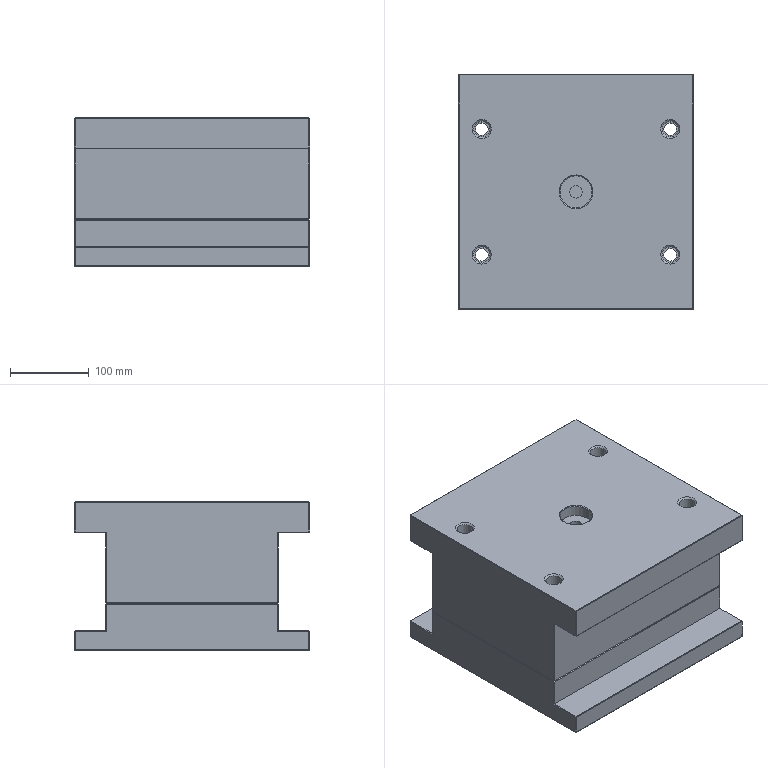NC program | NX | posted with a generic post | part box 300 x 300 x 190 mm
Lines 1 to 902 of 34829:
N10 G17 G21 G94 G90
(CAVITY_MILL_COPY_1 , TOOL : D25R5)
N12 T02 M6
N14 G54
N16 G17 G0 G90 X-7.201 Y-12.74 S1000 M3
N18 G43 Z30. H2
N20 Z1.5
N22 G94 G1 X-6.125 Y-13.304 Z1.436 F1000.
N24 X-4.712 Y-13.868 Z1.357
N26 X-3.248 Y-14.282 Z1.277
N28 X-2.184 Y-14.483 Z1.22
N30 X-1.089 Y-14.606 Z1.162
N32 X0.012 Y-14.646 Z1.105
N34 X1.113 Y-14.604 Z1.047
N36 X2.188 Y-14.482 Z0.99
N38 X3.607 Y-14.195 Z0.914
N40 X4.99 Y-13.77 Z0.838
N42 X6.325 Y-13.211 Z0.763
N44 X7.597 Y-12.522 Z0.687
N46 X8.796 Y-11.711 Z0.611
N48 X9.909 Y-10.786 Z0.535
N50 X10.925 Y-9.755 Z0.459
N52 X11.834 Y-8.629 Z0.383
N54 X12.628 Y-7.419 Z0.308
N56 X13.299 Y-6.137 Z0.232
N58 X13.839 Y-4.795 Z0.156
N60 X14.245 Y-3.405 Z0.08
N62 X14.512 Y-1.983 Z0.004
N64 X14.636 Y-0.541 Z-0.072
N66 Y0. Z-0.1
N68 X4.886
N70 G3 X0. Y4.886 R4.886 F2000.
N72 X4.886 Y0. R-4.886
N74 G1 X14.636
N76 G3 X0. Y14.636 R14.636
N78 X14.636 Y0. R-14.636
N80 G1 X24.386
N82 G3 X0. Y24.386 R24.386
N84 X24.386 Y0. R-24.386
N86 G1 X34.136
N88 G3 X0. Y34.136 R34.136
N90 X34.136 Y0. R-34.136
N92 G1 X43.886
N94 G3 X0. Y43.886 R43.886
N96 X43.886 Y0. R-43.886
N98 X43.386 Y0.866 R1.
N100 G1 Z1.4
N102 G0 X-11.531 Y-7.454
N104 G1 X-11.121 Y-8.085 Z1.361 F1000.
N106 X-10.205 Y-9.214 Z1.284
N108 X-9.175 Y-10.24 Z1.208
N110 X-8.042 Y-11.152 Z1.132
N112 X-6.819 Y-11.939 Z1.056
N114 X-5.52 Y-12.593 Z0.979
N116 X-4.159 Y-13.105 Z0.903
N118 X-2.751 Y-13.471 Z0.827
N120 X-1.716 Y-13.642 Z0.772
N122 X-0.443 Y-13.742 Z0.705
N124 X0.834 Y-13.724 Z0.638
N126 X1.877 Y-13.621 Z0.583
N128 X3.326 Y-13.341 Z0.506
N130 X4.736 Y-12.908 Z0.429
N132 X6.092 Y-12.326 Z0.351
N134 X7.378 Y-11.602 Z0.274
N136 X8.579 Y-10.745 Z0.197
N138 X9.681 Y-9.764 Z0.119
N140 X10.671 Y-8.67 Z0.042
N142 X11.539 Y-7.477 Z-0.035
N144 X12.273 Y-6.197 Z-0.113
N146 X12.867 Y-4.846 Z-0.19
N148 X13.312 Y-3.44 Z-0.267
N150 X13.604 Y-1.994 Z-0.345
N152 X13.739 Y-0.524 Z-0.422
N154 Y0. Z-0.449
N156 X3.989
N158 G3 X0. Y3.989 R3.989 F2000.
N160 X3.989 Y0. R-3.989
N162 G1 X13.739
N164 G3 X0. Y13.739 R13.739
N166 X13.739 Y0. R-13.739
N168 G1 X23.489
N170 G3 X0. Y23.489 R23.489
N172 X23.489 Y0. R-23.489
N174 G1 X33.239
N176 G3 X0. Y33.239 R33.239
N178 X33.239 Y0. R-33.239
N180 G1 X42.989
N182 G3 X0. Y42.989 R42.989
N184 X42.989 Y0. R-42.989
N186 X42.489 Y0.866 R1.
N188 G1 Z1.051
N190 G0 X11.782 Y5.822
N192 G1 X11.396 Y6.583 Z1.006 F1000.
N194 X10.849 Y7.45 Z0.952
N196 X9.981 Y8.578 Z0.878
N198 X8.997 Y9.605 Z0.803
N200 X7.908 Y10.52 Z0.728
N202 X6.726 Y11.312 Z0.654
N204 X5.466 Y11.972 Z0.579
N206 X4.142 Y12.492 Z0.505
N208 X2.769 Y12.866 Z0.43
N210 X1.364 Y13.09 Z0.356
N212 X-0.057 Y13.16 Z0.281
N214 X-1.477 Y13.077 Z0.207
N216 X-2.88 Y12.842 Z0.132
N218 X-4.249 Y12.456 Z0.057
N220 X-5.569 Y11.924 Z-0.017
N222 X-6.823 Y11.254 Z-0.092
N224 X-7.998 Y10.451 Z-0.166
N226 X-9.079 Y9.527 Z-0.241
N228 X-10.055 Y8.491 Z-0.315
N230 X-10.912 Y7.357 Z-0.39
N232 X-11.452 Y6.484 Z-0.444
N234 X-12.017 Y5.366 Z-0.509
N236 X-12.473 Y4.199 Z-0.575
N238 X-12.816 Y2.993 Z-0.641
N240 X-13.042 Y1.761 Z-0.706
N242 X-13.151 Y0.513 Z-0.772
N244 Y0. Z-0.799
N246 X-3.401
N248 G3 X0. Y-3.401 R3.401 F2000.
N250 X-3.401 Y0. R-3.401
N252 G1 X-13.151
N254 G3 X0. Y-13.151 R13.151
N256 X-13.151 Y0. R-13.151
N258 G1 X-22.901
N260 G3 X0. Y-22.901 R22.901
N262 X-22.901 Y0. R-22.901
N264 G1 X-32.651
N266 G3 X0. Y-32.651 R32.651
N268 X-32.651 Y0. R-32.651
N270 G1 X-42.401
N272 G3 X0. Y-42.401 R42.401
N274 X-42.401 Y0. R-42.401
N276 X-41.901 Y-0.866 R1.
N278 G1 Z0.701
N280 G0 X4.519 Y-11.874
N282 G1 X5.691 Y-11.364 Z0.634 F1000.
N284 X6.88 Y-10.686 Z0.562
N286 X7.99 Y-9.884 Z0.491
N288 X9.006 Y-8.967 Z0.419
N290 X9.919 Y-7.946 Z0.347
N292 X10.716 Y-6.833 Z0.275
N294 X11.389 Y-5.641 Z0.204
N296 X11.929 Y-4.383 Z0.132
N298 X12.332 Y-3.075 Z0.06
N300 X12.591 Y-1.731 Z-0.012
N302 X12.704 Y-0.366 Z-0.083
N304 X12.67 Y1.002 Z-0.155
N306 X12.488 Y2.359 Z-0.227
N308 X12.162 Y3.689 Z-0.299
N310 X11.695 Y4.976 Z-0.37
N312 X11.092 Y6.205 Z-0.442
N314 X10.565 Y7.064 Z-0.495
N316 X9.769 Y8.129 Z-0.565
N318 X8.867 Y9.105 Z-0.634
N320 X7.867 Y9.981 Z-0.704
N322 X6.782 Y10.749 Z-0.774
N324 X5.622 Y11.398 Z-0.843
N326 X4.401 Y11.923 Z-0.913
N328 X3.131 Y12.317 Z-0.983
N330 X1.828 Y12.577 Z-1.052
N332 X0.504 Y12.699 Z-1.122
N334 X0. Z-1.148
N336 Y2.949
N338 G3 X-2.949 Y0. R2.949 F2000.
N340 X0. Y2.949 R-2.949
N342 G1 Y12.699
N344 G3 X-12.699 Y0. R12.699
N346 X0. Y12.699 R-12.699
N348 G1 Y22.449
N350 G3 X-22.449 Y0. R22.449
N352 X0. Y22.449 R-22.449
N354 G1 Y32.199
N356 G3 X-32.199 Y0. R32.199
N358 X0. Y32.199 R-32.199
N360 G1 Y41.949
N362 G3 X-41.949 Y0. R41.949
N364 X0. Y41.949 R-41.949
N366 X-0.866 Y41.449 R1.
N368 G1 Z0.352
N370 G0 X3.427 Y-11.844
N372 G1 X4.33 Y-11.561 Z0.302 F1000.
N374 X5.55 Y-11.027 Z0.232
N376 X6.706 Y-10.365 Z0.163
N378 X7.783 Y-9.582 Z0.093
N380 X8.771 Y-8.687 Z0.023
N382 X9.656 Y-7.692 Z-0.047
N384 X10.428 Y-6.607 Z-0.117
N386 X11.079 Y-5.445 Z-0.187
N388 X11.601 Y-4.219 Z-0.256
N390 X11.988 Y-2.945 Z-0.326
N392 X12.236 Y-1.636 Z-0.396
N394 X12.341 Y-0.308 Z-0.466
N396 X12.302 Y1.024 Z-0.536
N398 X12.12 Y2.343 Z-0.605
N400 X11.797 Y3.635 Z-0.675
N402 X11.337 Y4.885 Z-0.745
N404 X10.745 Y6.078 Z-0.815
N406 X10.221 Y6.923 Z-0.867
N408 X9.448 Y7.946 Z-0.934
N410 X8.573 Y8.883 Z-1.001
N412 X7.605 Y9.724 Z-1.068
N414 X6.555 Y10.46 Z-1.136
N416 X5.435 Y11.084 Z-1.203
N418 X4.256 Y11.588 Z-1.27
N420 X3.031 Y11.967 Z-1.337
N422 X1.774 Y12.217 Z-1.404
N424 X0.497 Y12.335 Z-1.472
N426 X0. Z-1.498
N428 Y2.585
N430 G3 X-2.585 Y0. R2.585 F2000.
N432 X0. Y2.585 R-2.585
N434 G1 Y12.335
N436 G3 X-12.335 Y0. R12.335
N438 X0. Y12.335 R-12.335
N440 G1 Y22.085
N442 G3 X-22.085 Y0. R22.085
N444 X0. Y22.085 R-22.085
N446 G1 Y31.835
N448 G3 X-31.835 Y0. R31.835
N450 X0. Y31.835 R-31.835
N452 G1 Y41.585
N454 G3 X-41.585 Y0. R41.585
N456 X0. Y41.585 R-41.585
N458 X-0.866 Y41.085 R1.
N460 G1 Z0.002
N462 G0 X2.506 Y-11.76
N464 G1 X3.075 Y-11.644 Z-0.028 F1000.
N466 X4.384 Y-11.217 Z-0.1
N468 X5.637 Y-10.643 Z-0.172
N470 X6.816 Y-9.929 Z-0.245
N472 X7.905 Y-9.086 Z-0.317
N474 X8.891 Y-8.123 Z-0.389
N476 X9.761 Y-7.055 Z-0.461
N478 X10.503 Y-5.894 Z-0.534
N480 X11.107 Y-4.655 Z-0.606
N482 X11.566 Y-3.356 Z-0.678
N484 X11.874 Y-2.013 Z-0.75
N486 X12.026 Y-0.644 Z-0.822
N488 X12.021 Y0.734 Z-0.895
N490 X11.858 Y2.102 Z-0.967
N492 X11.541 Y3.443 Z-1.039
N494 X11.072 Y4.739 Z-1.111
N496 X10.458 Y5.972 Z-1.183
N498 X9.937 Y6.804 Z-1.235
N500 X9.183 Y7.792 Z-1.3
N502 X8.33 Y8.698 Z-1.365
N504 X7.389 Y9.51 Z-1.43
N506 X6.369 Y10.221 Z-1.496
N508 X5.281 Y10.824 Z-1.561
N510 X4.137 Y11.311 Z-1.626
N512 X2.949 Y11.677 Z-1.691
N514 X1.729 Y11.919 Z-1.756
N516 X0.491 Y12.033 Z-1.821
N518 X0. Z-1.847
N520 Y2.283
N522 G3 X-2.283 Y0. R2.283 F2000.
N524 X0. Y2.283 R-2.283
N526 G1 Y12.033
N528 G3 X-12.033 Y0. R12.033
N530 X0. Y12.033 R-12.033
N532 G1 Y21.783
N534 G3 X-21.783 Y0. R21.783
N536 X0. Y21.783 R-21.783
N538 G1 Y31.533
N540 G3 X-31.533 Y0. R31.533
N542 X0. Y31.533 R-31.533
N544 G1 Y41.283
N546 G3 X-41.283 Y0. R41.283
N548 X0. Y41.283 R-41.283
N550 X-0.866 Y40.783 R1.
N552 G1 Z-0.347
N554 G0 X1.73 Y-11.662
N556 G1 X3.024 Y-11.397 Z-0.416 F1000.
N558 X4.308 Y-10.977 Z-0.487
N560 X5.535 Y-10.412 Z-0.558
N562 X6.689 Y-9.711 Z-0.629
N564 X7.756 Y-8.882 Z-0.699
N566 X8.72 Y-7.937 Z-0.77
N568 X9.571 Y-6.888 Z-0.841
N570 X10.296 Y-5.748 Z-0.912
N572 X10.886 Y-4.533 Z-0.983
N574 X11.333 Y-3.258 Z-1.053
N576 X11.631 Y-1.941 Z-1.124
N578 X11.776 Y-0.598 Z-1.195
N580 X11.768 Y0.752 Z-1.266
N582 X11.604 Y2.093 Z-1.337
N584 X11.289 Y3.406 Z-1.407
N586 X10.825 Y4.675 Z-1.478
N588 X10.22 Y5.882 Z-1.549
N590 X9.701 Y6.703 Z-1.6
N592 X8.863 Y7.778 Z-1.671
N594 X7.907 Y8.748 Z-1.743
N596 X6.845 Y9.602 Z-1.814
N598 X5.691 Y10.327 Z-1.885
N600 X4.462 Y10.915 Z-1.957
N602 X3.173 Y11.357 Z-2.028
N604 X1.841 Y11.647 Z-2.1
N606 X0.486 Y11.782 Z-2.171
N608 X0. Z-2.196
N610 Y2.032
N612 G3 X-2.032 Y0. R2.032 F2000.
N614 X0. Y2.032 R-2.032
N616 G1 Y11.782
N618 G3 X-11.782 Y0. R11.782
N620 X0. Y11.782 R-11.782
N622 G1 Y21.532
N624 G3 X-21.532 Y0. R21.532
N626 X0. Y21.532 R-21.532
N628 G1 Y31.282
N630 G3 X-31.282 Y0. R31.282
N632 X0. Y31.282 R-31.282
N634 G1 Y41.032
N636 G3 X-41.032 Y0. R41.032
N638 X0. Y41.032 R-41.032
N640 X-0.866 Y40.532 R1.
N642 G1 Z-0.696
N644 G0 X-11.514 Y-1.073
N646 G1 X-11.463 Y-1.654 Z-0.727 F1000.
N648 X-11.208 Y-2.918 Z-0.795
N650 X-10.814 Y-4.146 Z-0.862
N652 X-10.286 Y-5.322 Z-0.93
N654 X-9.63 Y-6.433 Z-0.997
N656 X-8.856 Y-7.463 Z-1.065
N658 X-7.971 Y-8.402 Z-1.133
N660 X-6.987 Y-9.236 Z-1.2
N662 X-5.917 Y-9.955 Z-1.268
N664 X-4.774 Y-10.552 Z-1.335
N666 X-3.571 Y-11.017 Z-1.403
N668 X-2.324 Y-11.346 Z-1.47
N670 X-1.374 Y-11.499 Z-1.521
N672 X-0.427 Y-11.573 Z-1.571
N674 X0.523 Y-11.569 Z-1.62
N676 X1.481 Y-11.486 Z-1.671
N678 X2.809 Y-11.235 Z-1.742
N680 X4.099 Y-10.832 Z-1.813
N682 X5.333 Y-10.28 Z-1.883
N684 X6.494 Y-9.589 Z-1.954
N686 X7.567 Y-8.768 Z-2.025
N688 X8.536 Y-7.827 Z-2.096
N690 X9.39 Y-6.779 Z-2.167
N692 X10.116 Y-5.639 Z-2.237
N694 X10.704 Y-4.422 Z-2.308
N696 X11.146 Y-3.145 Z-2.379
N698 X11.436 Y-1.826 Z-2.45
N700 X11.571 Y-0.481 Z-2.521
N702 Y0. Z-2.546
N704 X1.821
N706 G3 X0. Y1.821 R1.821 F2000.
N708 X1.821 Y0. R-1.821
N710 G1 X11.571
N712 G3 X0. Y11.571 R11.571
N714 X11.571 Y0. R-11.571
N716 G1 X21.321
N718 G3 X0. Y21.321 R21.321
N720 X21.321 Y0. R-21.321
N722 G1 X31.071
N724 G3 X0. Y31.071 R31.071
N726 X31.071 Y0. R-31.071
N728 G1 X40.821
N730 G3 X0. Y40.821 R40.821
N732 X40.821 Y0. R-40.821
N734 X40.321 Y0.866 R1.
N736 G1 Z-1.046
N738 G0 X-11.39 Y-0.527
N740 G1 X-11.275 Y-1.726 Z-1.109 F1000.
N742 X-11.008 Y-2.989 Z-1.177
N744 X-10.6 Y-4.214 Z-1.244
N746 X-10.056 Y-5.385 Z-1.312
N748 X-9.383 Y-6.486 Z-1.38
N750 X-8.59 Y-7.505 Z-1.447
N752 X-7.686 Y-8.428 Z-1.515
N754 X-6.685 Y-9.242 Z-1.583
N756 X-5.598 Y-9.939 Z-1.65
N758 X-4.439 Y-10.507 Z-1.718
N760 X-3.223 Y-10.942 Z-1.786
N762 X-1.966 Y-11.236 Z-1.853
N764 X-1.019 Y-11.361 Z-1.903
N766 X-0.153 Y-11.405 Z-1.949
N768 X0.714 Y-11.384 Z-1.994
N770 X1.664 Y-11.284 Z-2.044
N772 X2.95 Y-11.018 Z-2.113
N774 X4.197 Y-10.606 Z-2.182
N776 X5.389 Y-10.053 Z-2.251
N778 X6.509 Y-9.367 Z-2.32
N780 X7.542 Y-8.557 Z-2.388
N782 X8.476 Y-7.633 Z-2.457
N784 X9.297 Y-6.608 Z-2.526
N786 X9.995 Y-5.496 Z-2.595
N788 X10.561 Y-4.31 Z-2.664
N790 X10.986 Y-3.068 Z-2.733
N792 X11.266 Y-1.784 Z-2.801
N794 X11.397 Y-0.478 Z-2.87
N796 Y0. Z-2.895
N798 X1.647
N800 G3 X0. Y1.647 R1.647 F2000.
N802 X1.647 Y0. R-1.647
N804 G1 X11.397
N806 G3 X0. Y11.397 R11.397
N808 X11.397 Y0. R-11.397
N810 G1 X21.147
N812 G3 X0. Y21.147 R21.147
N814 X21.147 Y0. R-21.147
N816 G1 X30.897
N818 G3 X0. Y30.897 R30.897
N820 X30.897 Y0. R-30.897
N822 G1 X40.647
N824 G3 X0. Y40.647 R40.647
N826 X40.647 Y0. R-40.647
N828 X40.147 Y0.866 R1.
N830 G1 Z-1.395
N832 G0 X11.246 Y0.079
N834 G1 X11.248 Y0.6 Z-1.423 F1000.
N836 X11.106 Y1.875 Z-1.49
N838 X10.821 Y3.125 Z-1.557
N840 X10.396 Y4.335 Z-1.624
N842 X9.836 Y5.488 Z-1.691
N844 X9.339 Y6.297 Z-1.741
N846 X8.564 Y7.317 Z-1.808
N848 X7.677 Y8.242 Z-1.875
N850 X6.692 Y9.06 Z-1.943
N852 X5.62 Y9.761 Z-2.01
N854 X4.475 Y10.336 Z-2.077
N856 X3.273 Y10.778 Z-2.144
N858 X2.028 Y11.08 Z-2.211
N860 X0.756 Y11.238 Z-2.278
N862 X-0.525 Y11.251 Z-2.345
N864 X-1.799 Y11.119 Z-2.413
N866 X-3.05 Y10.843 Z-2.48
N868 X-4.261 Y10.426 Z-2.547
N870 X-5.417 Y9.875 Z-2.614
N872 X-6.504 Y9.196 Z-2.681
N874 X-7.506 Y8.398 Z-2.748
N876 X-8.411 Y7.492 Z-2.815
N878 X-9.207 Y6.488 Z-2.883
N880 X-9.721 Y5.69 Z-2.932
N882 X-10.228 Y4.717 Z-2.99
N884 X-10.639 Y3.699 Z-3.047
N886 X-10.948 Y2.646 Z-3.105
N888 X-11.154 Y1.568 Z-3.162
N890 X-11.254 Y0.475 Z-3.22
N892 Y0. Z-3.245
N894 X-1.504
N896 G3 X0. Y-1.504 R1.504 F2000.
N898 X-1.504 Y0. R-1.504
N900 G1 X-11.254
N902 G3 X0. Y-11.254 R11.254
N904 X-11.254 Y0. R-11.254
N906 G1 X-21.004
N908 G3 X0. Y-21.004 R21.004
N910 X-21.004 Y0. R-21.004
N912 G1 X-30.754
N914 G3 X0. Y-30.754 R30.754
N916 X-30.754 Y0. R-30.754
N918 G1 X-40.504
N920 G3 X0. Y-40.504 R40.504
N922 X-40.504 Y0. R-40.504
N924 X-40.004 Y-0.866 R1.
N926 G1 Z-1.745
N928 G0 X-0.28 Y-11.135
N930 G1 X0.7 Y-11.128 Z-1.796 F1000.
N932 X1.639 Y-11.028 Z-1.846
N934 X2.881 Y-10.771 Z-1.912
N936 X4.084 Y-10.374 Z-1.978
N938 X5.236 Y-9.844 Z-2.045
N940 X6.319 Y-9.186 Z-2.111
N942 X7.321 Y-8.409 Z-2.178
N944 X8.228 Y-7.524 Z-2.244
N946 X9.029 Y-6.542 Z-2.311
N948 X9.713 Y-5.475 Z-2.377
N950 X10.272 Y-4.337 Z-2.443
N952 X10.697 Y-3.143 Z-2.51
N954 X10.985 Y-1.908 Z-2.576
N956 X11.131 Y-0.649 Z-2.643
N958 X11.132 Y0.618 Z-2.709
N960 X10.99 Y1.878 Z-2.776
N962 X10.706 Y3.113 Z-2.842
N964 X10.284 Y4.308 Z-2.908
N966 X9.728 Y5.448 Z-2.975
N968 X9.232 Y6.251 Z-3.024
N970 X8.442 Y7.283 Z-3.093
N972 X7.537 Y8.216 Z-3.161
N974 X6.529 Y9.038 Z-3.229
N976 X5.433 Y9.736 Z-3.297
N978 X4.263 Y10.302 Z-3.365
N980 X3.035 Y10.729 Z-3.433
N982 X1.765 Y11.009 Z-3.501
N984 X0.472 Y11.14 Z-3.569
N986 X0. Z-3.594
N988 Y1.39
N990 G3 X-1.39 Y0. R1.39 F2000.
N992 X0. Y1.39 R-1.39
N994 G1 Y11.14
N996 G3 X-11.14 Y0. R11.14
N998 X0. Y11.14 R-11.14
N1000 G1 Y20.89
N1002 G3 X-20.89 Y0. R20.89
N1004 X0. Y20.89 R-20.89
N1006 G1 Y30.64
N1008 G3 X-30.64 Y0. R30.64
N1010 X0. Y30.64 R-30.64
N1012 G1 Y40.39
N1014 G3 X-40.39 Y0. R40.39
N1016 X0. Y40.39 R-40.39
N1018 X-0.866 Y39.89 R1.
N1020 G1 Z-2.094
N1022 G0 X11.044 Y-0.552
N1024 G1 X11.045 Y0.624 Z-2.156 F1000.
N1026 X10.903 Y1.875 Z-2.222
N1028 X10.619 Y3.1 Z-2.288
N1030 X10.199 Y4.286 Z-2.354
N1032 X9.646 Y5.416 Z-2.42
N1034 X9.151 Y6.216 Z-2.469
N1036 X8.387 Y7.214 Z-2.535
N1038 X7.514 Y8.119 Z-2.601
N1040 X6.545 Y8.919 Z-2.666
N1042 X5.491 Y9.604 Z-2.732
N1044 X4.366 Y10.165 Z-2.798
N1046 X3.185 Y10.594 Z-2.864
N1048 X1.963 Y10.887 Z-2.93
N1050 X0.715 Y11.039 Z-2.996
N1052 X-0.542 Y11.049 Z-3.062
N1054 X-1.792 Y10.917 Z-3.128
N1056 X-3.018 Y10.643 Z-3.193
N1058 X-4.206 Y10.232 Z-3.259
N1060 X-5.34 Y9.689 Z-3.325
N1062 X-6.404 Y9.02 Z-3.391
N1064 X-7.386 Y8.236 Z-3.457
N1066 X-8.273 Y7.345 Z-3.523
N1068 X-9.052 Y6.359 Z-3.589
N1070 X-9.56 Y5.567 Z-3.638
N1072 X-10.054 Y4.615 Z-3.694
N1074 X-10.453 Y3.62 Z-3.75
N1076 X-10.755 Y2.591 Z-3.807
N1078 X-10.955 Y1.538 Z-3.863
N1080 X-11.053 Y0.47 Z-3.919
N1082 Y0. Z-3.944
N1084 X-1.303
N1086 G3 X0. Y-1.303 R1.303 F2000.
N1088 X-1.303 Y0. R-1.303
N1090 G1 X-11.053
N1092 G3 X0. Y-11.053 R11.053
N1094 X-11.053 Y0. R-11.053
N1096 G1 X-20.803
N1098 G3 X0. Y-20.803 R20.803
N1100 X-20.803 Y0. R-20.803
N1102 G1 X-30.553
N1104 G3 X0. Y-30.553 R30.553
N1106 X-30.553 Y0. R-30.553
N1108 G1 X-40.303
N1110 G3 X0. Y-40.303 R40.303
N1112 X-40.303 Y0. R-40.303
N1114 X-39.803 Y-0.866 R1.
N1116 G1 Z-2.444
N1118 G0 X10.97 Y-0.745
N1120 G1 X10.984 Y-0.623 Z-2.45 F1000.
N1122 X10.983 Y0.629 Z-2.516
N1124 X10.841 Y1.872 Z-2.581
N1126 X10.558 Y3.091 Z-2.647
N1128 X10.139 Y4.27 Z-2.712
N1130 X9.588 Y5.394 Z-2.778
N1132 X9.094 Y6.191 Z-2.827
N1134 X8.327 Y7.19 Z-2.893
N1136 X7.451 Y8.094 Z-2.959
N1138 X6.478 Y8.892 Z-3.025
N1140 X5.42 Y9.574 Z-3.091
N1142 X4.291 Y10.13 Z-3.157
N1144 X3.106 Y10.554 Z-3.223
N1146 X1.88 Y10.839 Z-3.289
N1148 X0.629 Y10.983 Z-3.355
N1150 X-0.629 Z-3.421
N1152 X-1.88 Y10.839 Z-3.487
N1154 X-3.106 Y10.554 Z-3.553
N1156 X-4.291 Y10.13 Z-3.619
N1158 X-5.42 Y9.574 Z-3.685
N1160 X-6.478 Y8.892 Z-3.751
N1162 X-7.451 Y8.094 Z-3.817
N1164 X-8.327 Y7.19 Z-3.883
N1166 X-9.094 Y6.191 Z-3.949
N1168 X-9.588 Y5.394 Z-3.998
N1170 X-10.154 Y4.234 Z-4.065
N1172 X-10.58 Y3.014 Z-4.133
N1174 X-10.861 Y1.754 Z-4.201
N1176 X-10.991 Y0.469 Z-4.268
N1178 Y0. Z-4.293
N1180 X-1.241
N1182 G3 X0. Y-1.241 R1.241 F2000.
N1184 X-1.241 Y0. R-1.241
N1186 G1 X-10.991
N1188 G3 X0. Y-10.991 R10.991
N1190 X-10.991 Y0. R-10.991
N1192 G1 X-20.741
N1194 G3 X0. Y-20.741 R20.741
N1196 X-20.741 Y0. R-20.741
N1198 G1 X-30.491
N1200 G3 X0. Y-30.491 R30.491
N1202 X-30.491 Y0. R-30.491
N1204 G1 X-40.241
N1206 G3 X0. Y-40.241 R40.241
N1208 X-40.241 Y0. R-40.241
N1210 X-39.741 Y-0.866 R1.
N1212 G1 Z-2.793
N1214 G0 X-0.859 Y-10.918
N1216 G1 X-0.381 Y-10.958 Z-2.818 F1000.
N1218 X0.69 Y-10.943 Z-2.874
N1220 X1.621 Y-10.844 Z-2.923
N1222 X2.843 Y-10.59 Z-2.989
N1224 X4.027 Y-10.198 Z-3.054
N1226 X5.16 Y-9.675 Z-3.12
N1228 X6.225 Y-9.026 Z-3.185
N1230 X7.21 Y-8.26 Z-3.25
N1232 X8.102 Y-7.388 Z-3.316
N1234 X8.889 Y-6.42 Z-3.381
N1236 X9.56 Y-5.368 Z-3.446
N1238 X10.108 Y-4.247 Z-3.512
N1240 X10.525 Y-3.072 Z-3.577
N1242 X10.806 Y-1.856 Z-3.643
N1244 X10.947 Y-0.616 Z-3.708
N1246 X10.946 Y0.631 Z-3.773
N1248 X10.804 Y1.871 Z-3.839
N1250 X10.521 Y3.086 Z-3.904
N1252 X10.103 Y4.261 Z-3.969
N1254 X9.553 Y5.381 Z-4.035
N1256 X9.059 Y6.176 Z-4.084
N1258 X8.282 Y7.185 Z-4.151
N1260 X7.393 Y8.097 Z-4.217
N1262 X6.404 Y8.9 Z-4.284
N1264 X5.329 Y9.582 Z-4.351
N1266 X4.182 Y10.136 Z-4.418
N1268 X2.979 Y10.552 Z-4.484
N1270 X1.735 Y10.826 Z-4.551
N1272 X0.468 Y10.955 Z-4.618
N1274 X0. Z-4.642
N1276 Y1.205
N1278 G3 X-1.205 Y0. R1.205 F2000.
N1280 X0. Y1.205 R-1.205
N1282 G1 Y10.955
N1284 G3 X-10.955 Y0. R10.955
N1286 X0. Y10.955 R-10.955
N1288 G1 Y20.705
N1290 G3 X-20.705 Y0. R20.705
N1292 X0. Y20.705 R-20.705
N1294 G1 Y30.455
N1296 G3 X-30.455 Y0. R30.455
N1298 X0. Y30.455 R-30.455
N1300 G1 Y40.205
N1302 G3 X-40.205 Y0. R40.205
N1304 X0. Y40.205 R-40.205
N1306 X-0.866 Y39.705 R1.
N1308 G1 Z-3.142
N1310 G0 X0.898 Y10.898
N1312 G1 X0.11 Y10.951 Z-3.184 F1000.
N1314 X-1.154 Y10.891 Z-3.25
N1316 X-2.402 Y10.685 Z-3.316
N1318 X-3.619 Y10.337 Z-3.383
N1320 X-4.787 Y9.85 Z-3.449
N1322 X-5.892 Y9.232 Z-3.515
N1324 X-6.917 Y8.491 Z-3.582
N1326 X-7.85 Y7.637 Z-3.648
N1328 X-8.679 Y6.68 Z-3.714
N1330 X-9.392 Y5.634 Z-3.781
N1332 X-9.979 Y4.513 Z-3.847
N1334 X-10.433 Y3.332 Z-3.913
N1336 X-10.748 Y2.106 Z-3.98
N1338 X-10.919 Y0.853 Z-4.046
N1340 X-10.952 Y-0.083 Z-4.095
N1342 X-10.874 Y-1.303 Z-4.159
N1344 X-10.661 Y-2.508 Z-4.223
N1346 X-10.315 Y-3.681 Z-4.287
N1348 X-9.84 Y-4.808 Z-4.351
N1350 X-9.243 Y-5.875 Z-4.416
N1352 X-8.53 Y-6.869 Z-4.48
N1354 X-7.711 Y-7.777 Z-4.544
N1356 X-6.796 Y-8.589 Z-4.608
N1358 X-5.796 Y-9.293 Z-4.672
N1360 X-4.981 Y-9.754 Z-4.721
N1362 X-3.907 Y-10.231 Z-4.783
N1364 X-2.789 Y-10.591 Z-4.844
N1366 X-1.638 Y-10.829 Z-4.906
N1368 X-0.468 Y-10.942 Z-4.967
N1370 X0. Z-4.992
N1372 Y-1.192
N1374 G3 X1.192 Y0. R1.192 F2000.
N1376 X0. Y-1.192 R-1.192
N1378 G1 Y-10.942
N1380 G3 X10.942 Y0. R10.942
N1382 X0. Y-10.942 R-10.942
N1384 G1 Y-20.692
N1386 G3 X20.692 Y0. R20.692
N1388 X0. Y-20.692 R-20.692
N1390 G1 Y-30.442
N1392 G3 X30.442 Y0. R30.442
N1394 X0. Y-30.442 R-30.442
N1396 G1 Y-40.192
N1398 G3 X40.192 Y0. R40.192
N1400 X0. Y-40.192 R-40.192
N1402 X0.866 Y-39.692 R1.
N1404 G1 Z-3.492
N1406 G0 X-10.899 Y0.899
N1408 G1 X-10.94 Y0.506 Z-3.513 F1000.
N1410 X-10.925 Y-0.772 Z-3.58
N1412 X-10.76 Y-2.039 Z-3.646
N1414 X-10.45 Y-3.279 Z-3.713
N1416 X-9.997 Y-4.474 Z-3.78
N1418 X-9.408 Y-5.608 Z-3.847
N1420 X-8.69 Y-6.665 Z-3.914
N1422 X-7.855 Y-7.632 Z-3.981
N1424 X-6.912 Y-8.495 Z-4.048
N1426 X-5.876 Y-9.242 Z-4.115
N1428 X-4.759 Y-9.864 Z-4.182
N1430 X-3.578 Y-10.351 Z-4.249
N1432 X-2.348 Y-10.697 Z-4.316
N1434 X-1.426 Y-10.859 Z-4.365
N1436 X-0.37 Y-10.946 Z-4.421
N1438 X0.689 Y-10.93 Z-4.476
N1440 X1.62 Y-10.831 Z-4.525
N1442 X2.852 Y-10.574 Z-4.591
N1444 X4.046 Y-10.177 Z-4.657
N1446 X5.187 Y-9.646 Z-4.723
N1448 X6.259 Y-8.987 Z-4.789
N1450 X7.249 Y-8.21 Z-4.855
N1452 X8.143 Y-7.324 Z-4.921
N1454 X8.929 Y-6.342 Z-4.987
N1456 X9.598 Y-5.276 Z-5.053
N1458 X10.139 Y-4.14 Z-5.119
N1460 X10.547 Y-2.949 Z-5.185
N1462 X10.816 Y-1.72 Z-5.251
N1464 X10.942 Y-0.468 Z-5.317
N1466 Y0. Z-5.341
N1468 X1.192
N1470 G3 X0. Y1.192 R1.192 F2000.
N1472 X1.192 Y0. R-1.192
N1474 G1 X10.942
N1476 G3 X0. Y10.942 R10.942
N1478 X10.942 Y0. R-10.942
N1480 G1 X20.692
N1482 G3 X0. Y20.692 R20.692
N1484 X20.692 Y0. R-20.692
N1486 G1 X30.442
N1488 G3 X0. Y30.442 R30.442
N1490 X30.442 Y0. R-30.442
N1492 G1 X40.192
N1494 G3 X0. Y40.192 R40.192
N1496 X40.192 Y0. R-40.192
N1498 X39.692 Y0.866 R1.
N1500 G1 Z-3.841
N1502 G0 X-10.899 Y0.899
N1504 G1 X-10.94 Y0.506 Z-3.862 F1000.
N1506 X-10.925 Y-0.772 Z-3.929
N1508 X-10.76 Y-2.039 Z-3.996
N1510 X-10.45 Y-3.279 Z-4.063
N1512 X-9.997 Y-4.474 Z-4.13
N1514 X-9.408 Y-5.608 Z-4.197
N1516 X-8.69 Y-6.665 Z-4.264
N1518 X-7.855 Y-7.632 Z-4.331
N1520 X-6.912 Y-8.495 Z-4.398
N1522 X-5.876 Y-9.242 Z-4.465
N1524 X-4.759 Y-9.864 Z-4.532
N1526 X-3.578 Y-10.351 Z-4.599
N1528 X-2.348 Y-10.697 Z-4.666
N1530 X-1.426 Y-10.859 Z-4.715
N1532 X-0.37 Y-10.946 Z-4.77
N1534 X0.689 Y-10.93 Z-4.826
N1536 X1.62 Y-10.831 Z-4.875
N1538 X2.852 Y-10.574 Z-4.941
N1540 X4.046 Y-10.177 Z-5.007
N1542 X5.187 Y-9.646 Z-5.073
N1544 X6.259 Y-8.987 Z-5.139
N1546 X7.249 Y-8.21 Z-5.204
N1548 X8.143 Y-7.324 Z-5.27
N1550 X8.929 Y-6.342 Z-5.336
N1552 X9.598 Y-5.276 Z-5.402
N1554 X10.139 Y-4.14 Z-5.468
N1556 X10.547 Y-2.949 Z-5.534
N1558 X10.816 Y-1.72 Z-5.6
N1560 X10.942 Y-0.468 Z-5.666
N1562 Y0. Z-5.691
N1564 X1.192
N1566 G3 X0. Y1.192 R1.192 F2000.
N1568 X1.192 Y0. R-1.192
N1570 G1 X10.942
N1572 G3 X0. Y10.942 R10.942
N1574 X10.942 Y0. R-10.942
N1576 G1 X20.692
N1578 G3 X0. Y20.692 R20.692
N1580 X20.692 Y0. R-20.692
N1582 G1 X30.442
N1584 G3 X0. Y30.442 R30.442
N1586 X30.442 Y0. R-30.442
N1588 G1 X40.192
N1590 G3 X0. Y40.192 R40.192
N1592 X40.192 Y0. R-40.192
N1594 X39.692 Y0.866 R1.
N1596 G1 Z-4.191
N1598 G0 X-10.899 Y0.899
N1600 G1 X-10.94 Y0.506 Z-4.211 F1000.
N1602 X-10.925 Y-0.772 Z-4.278
N1604 X-10.76 Y-2.039 Z-4.345
N1606 X-10.45 Y-3.279 Z-4.412
N1608 X-9.997 Y-4.474 Z-4.479
N1610 X-9.408 Y-5.608 Z-4.546
N1612 X-8.69 Y-6.665 Z-4.613
N1614 X-7.855 Y-7.632 Z-4.68
N1616 X-6.912 Y-8.495 Z-4.747
N1618 X-5.876 Y-9.242 Z-4.814
N1620 X-4.759 Y-9.864 Z-4.881
N1622 X-3.578 Y-10.351 Z-4.948
N1624 X-2.348 Y-10.697 Z-5.015
N1626 X-1.426 Y-10.859 Z-5.064
N1628 X-0.37 Y-10.946 Z-5.12
N1630 X0.689 Y-10.93 Z-5.175
N1632 X1.62 Y-10.831 Z-5.224
N1634 X2.852 Y-10.574 Z-5.29
N1636 X4.046 Y-10.177 Z-5.356
N1638 X5.187 Y-9.646 Z-5.422
N1640 X6.259 Y-8.987 Z-5.488
N1642 X7.249 Y-8.21 Z-5.554
N1644 X8.143 Y-7.324 Z-5.62
N1646 X8.929 Y-6.342 Z-5.686
N1648 X9.598 Y-5.276 Z-5.752
N1650 X10.139 Y-4.14 Z-5.818
N1652 X10.547 Y-2.949 Z-5.884
N1654 X10.816 Y-1.72 Z-5.95
N1656 X10.942 Y-0.468 Z-6.016
N1658 Y0. Z-6.04
N1660 X1.192
N1662 G3 X0. Y1.192 R1.192 F2000.
N1664 X1.192 Y0. R-1.192
N1666 G1 X10.942
N1668 G3 X0. Y10.942 R10.942
N1670 X10.942 Y0. R-10.942
N1672 G1 X20.692
N1674 G3 X0. Y20.692 R20.692
N1676 X20.692 Y0. R-20.692
N1678 G1 X30.442
N1680 G3 X0. Y30.442 R30.442
N1682 X30.442 Y0. R-30.442
N1684 G1 X40.192
N1686 G3 X0. Y40.192 R40.192
N1688 X40.192 Y0. R-40.192
N1690 X39.692 Y0.866 R1.
N1692 G1 Z-4.54
N1694 G0 X-10.899 Y0.899
N1696 G1 X-10.94 Y0.506 Z-4.561 F1000.
N1698 X-10.925 Y-0.772 Z-4.628
N1700 X-10.76 Y-2.039 Z-4.695
N1702 X-10.45 Y-3.279 Z-4.762
N1704 X-9.997 Y-4.474 Z-4.829
N1706 X-9.408 Y-5.608 Z-4.896
N1708 X-8.69 Y-6.665 Z-4.963
N1710 X-7.855 Y-7.632 Z-5.03
N1712 X-6.912 Y-8.495 Z-5.097
N1714 X-5.876 Y-9.242 Z-5.163
N1716 X-4.759 Y-9.864 Z-5.23
N1718 X-3.578 Y-10.351 Z-5.297
N1720 X-2.348 Y-10.697 Z-5.364
N1722 X-1.426 Y-10.859 Z-5.413
N1724 X-0.37 Y-10.946 Z-5.469
N1726 X0.689 Y-10.93 Z-5.525
N1728 X1.62 Y-10.831 Z-5.574
N1730 X2.852 Y-10.574 Z-5.64
N1732 X4.046 Y-10.177 Z-5.705
N1734 X5.187 Y-9.646 Z-5.771
N1736 X6.259 Y-8.987 Z-5.837
N1738 X7.249 Y-8.21 Z-5.903
N1740 X8.143 Y-7.324 Z-5.969
N1742 X8.929 Y-6.342 Z-6.035
N1744 X9.598 Y-5.276 Z-6.101
N1746 X10.139 Y-4.14 Z-6.167
N1748 X10.547 Y-2.949 Z-6.233
N1750 X10.816 Y-1.72 Z-6.299
N1752 X10.942 Y-0.468 Z-6.365
N1754 Y0. Z-6.389
N1756 X1.192
N1758 G3 X0. Y1.192 R1.192 F2000.
N1760 X1.192 Y0. R-1.192
N1762 G1 X10.942
N1764 G3 X0. Y10.942 R10.942
N1766 X10.942 Y0. R-10.942
N1768 G1 X20.692
N1770 G3 X0. Y20.692 R20.692
N1772 X20.692 Y0. R-20.692
N1774 G1 X30.442
N1776 G3 X0. Y30.442 R30.442
N1778 X30.442 Y0. R-30.442
N1780 G1 X40.192
N1782 G3 X0. Y40.192 R40.192
N1784 X40.192 Y0. R-40.192
N1786 X39.692 Y0.866 R1.
N1788 G1 Z-4.889
N1790 G0 X-10.899 Y0.899
N1792 G1 X-10.94 Y0.506 Z-4.91 F1000.
N1794 X-10.925 Y-0.772 Z-4.977
N1796 X-10.76 Y-2.039 Z-5.044
N1798 X-10.45 Y-3.279 Z-5.111
N1800 X-9.997 Y-4.474 Z-5.178
N1802 X-9.408 Y-5.608 Z-5.245